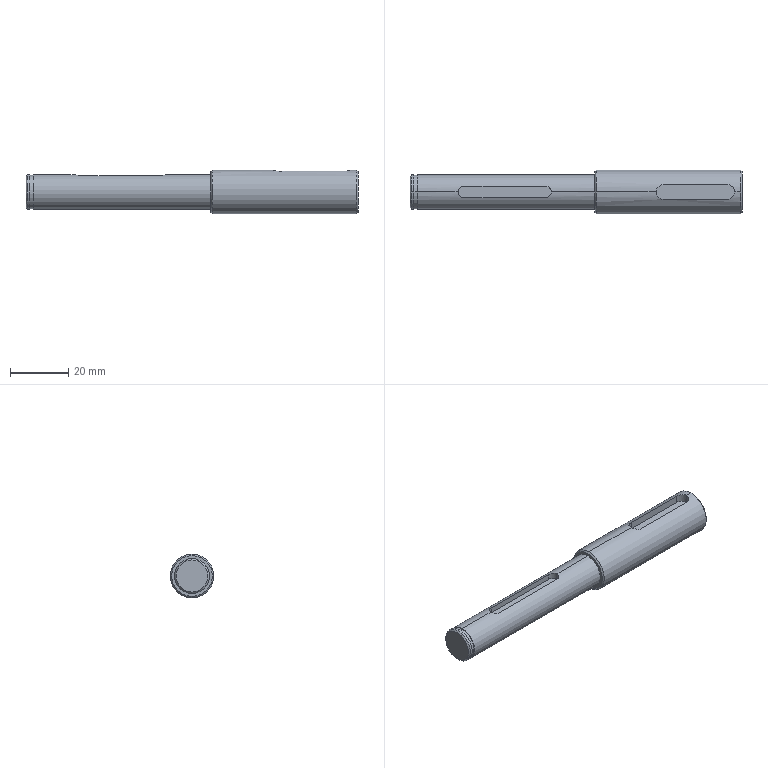Part | SolidWorks | features BaseBody 1 | 1 solid | 31 faces | box 114 x 15 x 15 mm | volume 15429 mm3 | cylinder 14 | plane 11 | cone 6 | commonest cylinder face diameters 12 x4 4 x3 5 x3 11.5 x2 15 x2
STEP:
#1=CARTESIAN_POINT('',(113.5,0.,7.5));
#2=VERTEX_POINT('',#1);
#3=CARTESIAN_POINT('',(113.5,0.,-7.5));
#4=VERTEX_POINT('',#3);
#5=CARTESIAN_POINT('',(113.5,0.,0.));
#6=DIRECTION('',(-1.,0.,0.));
#7=DIRECTION('',(0.,0.,1.));
#8=AXIS2_PLACEMENT_3D('',#5,#6,#7);
#9=CIRCLE('',#8,7.5);
#10=EDGE_CURVE('',#2,#4,#9,.T.);
#11=ORIENTED_EDGE('',*,*,#10,.T.);
#12=CARTESIAN_POINT('',(64.,0.,-7.5));
#13=VERTEX_POINT('',#12);
#14=CARTESIAN_POINT('',(0.,0.,-7.5));
#15=DIRECTION('',(-1.,0.,0.));
#16=VECTOR('',#15,1000.);
#17=LINE('',#14,#16);
#18=EDGE_CURVE('',#4,#13,#17,.T.);
#19=ORIENTED_EDGE('',*,*,#18,.T.);
#20=CARTESIAN_POINT('',(64.,0.,7.5));
#21=VERTEX_POINT('',#20);
#22=CARTESIAN_POINT('',(64.,0.,0.));
#23=DIRECTION('',(1.,0.,0.));
#24=DIRECTION('',(0.,0.,1.));
#25=AXIS2_PLACEMENT_3D('',#22,#23,#24);
#26=CIRCLE('',#25,7.5);
#27=EDGE_CURVE('',#13,#21,#26,.T.);
#28=ORIENTED_EDGE('',*,*,#27,.T.);
#29=CARTESIAN_POINT('',(84.5,0.,7.5));
#30=VERTEX_POINT('',#29);
#31=CARTESIAN_POINT('',(0.,0.,7.5));
#32=DIRECTION('',(-1.,0.,0.));
#33=VECTOR('',#32,1000.);
#34=LINE('',#31,#33);
#35=EDGE_CURVE('',#30,#21,#34,.T.);
#36=ORIENTED_EDGE('',*,*,#35,.F.);
#37=CARTESIAN_POINT('',(87.,2.5,7.071));
#38=VERTEX_POINT('',#37);
#39=CARTESIAN_POINT('',(84.5,0.,7.5));
#40=CARTESIAN_POINT('',(84.5,0.1664,7.5));
#41=CARTESIAN_POINT('',(84.516,0.3297,7.494));
#42=CARTESIAN_POINT('',(84.581,0.6507,7.473));
#43=CARTESIAN_POINT('',(84.629,0.8101,7.458));
#44=CARTESIAN_POINT('',(84.755,1.112,7.419));
#45=CARTESIAN_POINT('',(84.832,1.255,7.395));
#46=CARTESIAN_POINT('',(85.013,1.526,7.344));
#47=CARTESIAN_POINT('',(85.118,1.653,7.316));
#48=CARTESIAN_POINT('',(85.461,1.996,7.233));
#49=CARTESIAN_POINT('',(85.737,2.182,7.177));
#50=CARTESIAN_POINT('',(86.187,2.37,7.116));
#51=CARTESIAN_POINT('',(86.346,2.419,7.099));
#52=CARTESIAN_POINT('',(86.67,2.484,7.077));
#53=CARTESIAN_POINT('',(86.834,2.5,7.071));
#54=CARTESIAN_POINT('',(87.,2.5,7.071));
#55=B_SPLINE_CURVE_WITH_KNOTS('',3,(#39,#40,#41,#42,#43,#44,#45,#46,#47,#48,#49,#50,#51,#52,#53,#54),.UNSPECIFIED.,.F.,.F.,(4,2,2,2,2,2,2,4),(0.003934,0.004426,0.004917,0.005409,0.005901,0.006884,0.007376,0.007868),.UNSPECIFIED.);
#56=EDGE_CURVE('',#30,#38,#55,.T.);
#57=ORIENTED_EDGE('',*,*,#56,.T.);
#58=CARTESIAN_POINT('',(109.,2.5,7.071));
#59=VERTEX_POINT('',#58);
#60=CARTESIAN_POINT('',(0.,2.5,7.071));
#61=DIRECTION('',(1.,0.,0.));
#62=VECTOR('',#61,1000.);
#63=LINE('',#60,#62);
#64=EDGE_CURVE('',#38,#59,#63,.T.);
#65=ORIENTED_EDGE('',*,*,#64,.T.);
#66=CARTESIAN_POINT('',(111.5,0.,7.5));
#67=VERTEX_POINT('',#66);
#68=CARTESIAN_POINT('',(109.,2.5,7.071));
#69=CARTESIAN_POINT('',(109.166,2.5,7.071));
#70=CARTESIAN_POINT('',(109.33,2.484,7.077));
#71=CARTESIAN_POINT('',(109.651,2.419,7.099));
#72=CARTESIAN_POINT('',(109.81,2.371,7.116));
#73=CARTESIAN_POINT('',(110.112,2.245,7.156));
#74=CARTESIAN_POINT('',(110.255,2.168,7.18));
#75=CARTESIAN_POINT('',(110.526,1.987,7.233));
#76=CARTESIAN_POINT('',(110.653,1.883,7.261));
#77=CARTESIAN_POINT('',(110.996,1.54,7.344));
#78=CARTESIAN_POINT('',(111.182,1.263,7.399));
#79=CARTESIAN_POINT('',(111.37,0.8128,7.457));
#80=CARTESIAN_POINT('',(111.418,0.6543,7.473));
#81=CARTESIAN_POINT('',(111.484,0.3305,7.494));
#82=CARTESIAN_POINT('',(111.5,0.1664,7.5));
#83=CARTESIAN_POINT('',(111.5,0.,7.5));
#84=B_SPLINE_CURVE_WITH_KNOTS('',3,(#68,#69,#70,#71,#72,#73,#74,#75,#76,#77,#78,#79,#80,#81,#82,#83),.UNSPECIFIED.,.F.,.F.,(4,2,2,2,2,2,2,4),(-0.003934,-0.003442,-0.00295,-0.002459,-0.001967,-0.0009835,-0.0004917,0.),.UNSPECIFIED.);
#85=EDGE_CURVE('',#59,#67,#84,.T.);
#86=ORIENTED_EDGE('',*,*,#85,.T.);
#87=CARTESIAN_POINT('',(0.,0.,7.5));
#88=DIRECTION('',(-1.,0.,0.));
#89=VECTOR('',#88,1000.);
#90=LINE('',#87,#89);
#91=EDGE_CURVE('',#2,#67,#90,.T.);
#92=ORIENTED_EDGE('',*,*,#91,.F.);
#93=EDGE_LOOP('',(#11,#19,#28,#36,#57,#65,#86,#92));
#94=FACE_OUTER_BOUND('',#93,.T.);
#95=CARTESIAN_POINT('',(0.,0.,0.));
#96=DIRECTION('',(-1.,0.,0.));
#97=DIRECTION('',(0.,0.,1.));
#98=AXIS2_PLACEMENT_3D('',#95,#96,#97);
#99=CYLINDRICAL_SURFACE('',#98,7.5);
#100=ADVANCED_FACE('',(#94),#99,.T.);
#101=CARTESIAN_POINT('',(63.5,0.,-7.));
#102=VERTEX_POINT('',#101);
#103=CARTESIAN_POINT('',(63.5,0.,7.));
#104=VERTEX_POINT('',#103);
#105=CARTESIAN_POINT('',(63.5,0.,0.));
#106=DIRECTION('',(1.,0.,0.));
#107=DIRECTION('',(0.,0.,-1.));
#108=AXIS2_PLACEMENT_3D('',#105,#106,#107);
#109=CIRCLE('',#108,7.);
#110=EDGE_CURVE('',#102,#104,#109,.T.);
#111=ORIENTED_EDGE('',*,*,#110,.T.);
#112=CARTESIAN_POINT('',(64.,0.,7.5));
#113=DIRECTION('',(0.7071,0.,0.7071));
#114=VECTOR('',#113,1000.);
#115=LINE('',#112,#114);
#116=EDGE_CURVE('',#104,#21,#115,.T.);
#117=ORIENTED_EDGE('',*,*,#116,.T.);
#118=ORIENTED_EDGE('',*,*,#27,.F.);
#119=CARTESIAN_POINT('',(64.,0.,-7.5));
#120=DIRECTION('',(0.7071,0.,-0.7071));
#121=VECTOR('',#120,1000.);
#122=LINE('',#119,#121);
#123=EDGE_CURVE('',#102,#13,#122,.T.);
#124=ORIENTED_EDGE('',*,*,#123,.F.);
#125=EDGE_LOOP('',(#111,#117,#118,#124));
#126=FACE_OUTER_BOUND('',#125,.T.);
#127=CARTESIAN_POINT('',(64.,0.,0.));
#128=DIRECTION('',(1.,0.,0.));
#129=DIRECTION('',(0.,0.,-1.));
#130=AXIS2_PLACEMENT_3D('',#127,#128,#129);
#131=CONICAL_SURFACE('',#130,7.5,0.7854);
#132=ADVANCED_FACE('',(#126),#131,.T.);
#133=CARTESIAN_POINT('',(111.5,0.,4.5));
#134=VERTEX_POINT('',#133);
#135=CARTESIAN_POINT('',(109.,2.5,4.5));
#136=VERTEX_POINT('',#135);
#137=CARTESIAN_POINT('',(109.,0.,4.5));
#138=DIRECTION('',(0.,0.,1.));
#139=DIRECTION('',(1.,0.,0.));
#140=AXIS2_PLACEMENT_3D('',#137,#138,#139);
#141=CIRCLE('',#140,2.5);
#142=EDGE_CURVE('',#134,#136,#141,.T.);
#143=ORIENTED_EDGE('',*,*,#142,.F.);
#144=CARTESIAN_POINT('',(111.5,0.,4.5));
#145=DIRECTION('',(0.,0.,1.));
#146=VECTOR('',#145,1000.);
#147=LINE('',#144,#146);
#148=EDGE_CURVE('',#134,#67,#147,.T.);
#149=ORIENTED_EDGE('',*,*,#148,.T.);
#150=ORIENTED_EDGE('',*,*,#85,.F.);
#151=CARTESIAN_POINT('',(109.,2.5,4.5));
#152=DIRECTION('',(0.,0.,1.));
#153=VECTOR('',#152,1000.);
#154=LINE('',#151,#153);
#155=EDGE_CURVE('',#136,#59,#154,.T.);
#156=ORIENTED_EDGE('',*,*,#155,.F.);
#157=EDGE_LOOP('',(#143,#149,#150,#156));
#158=FACE_OUTER_BOUND('',#157,.T.);
#159=CARTESIAN_POINT('',(109.,0.,4.5));
#160=DIRECTION('',(0.,0.,1.));
#161=DIRECTION('',(1.,0.,0.));
#162=AXIS2_PLACEMENT_3D('',#159,#160,#161);
#163=CYLINDRICAL_SURFACE('',#162,2.5);
#164=ADVANCED_FACE('',(#158),#163,.F.);
#165=CARTESIAN_POINT('',(114.,0.,7.));
#166=VERTEX_POINT('',#165);
#167=CARTESIAN_POINT('',(114.,0.,-7.));
#168=VERTEX_POINT('',#167);
#169=CARTESIAN_POINT('',(114.,0.,0.));
#170=DIRECTION('',(-1.,0.,0.));
#171=DIRECTION('',(0.,0.,1.));
#172=AXIS2_PLACEMENT_3D('',#169,#170,#171);
#173=CIRCLE('',#172,7.);
#174=EDGE_CURVE('',#166,#168,#173,.T.);
#175=ORIENTED_EDGE('',*,*,#174,.T.);
#176=CARTESIAN_POINT('',(113.5,0.,-7.5));
#177=DIRECTION('',(-0.7071,0.,-0.7071));
#178=VECTOR('',#177,1000.);
#179=LINE('',#176,#178);
#180=EDGE_CURVE('',#168,#4,#179,.T.);
#181=ORIENTED_EDGE('',*,*,#180,.T.);
#182=ORIENTED_EDGE('',*,*,#10,.F.);
#183=CARTESIAN_POINT('',(113.5,0.,7.5));
#184=DIRECTION('',(-0.7071,0.,0.7071));
#185=VECTOR('',#184,1000.);
#186=LINE('',#183,#185);
#187=EDGE_CURVE('',#166,#2,#186,.T.);
#188=ORIENTED_EDGE('',*,*,#187,.F.);
#189=EDGE_LOOP('',(#175,#181,#182,#188));
#190=FACE_OUTER_BOUND('',#189,.T.);
#191=CARTESIAN_POINT('',(113.5,0.,0.));
#192=DIRECTION('',(-1.,0.,0.));
#193=DIRECTION('',(0.,0.,1.));
#194=AXIS2_PLACEMENT_3D('',#191,#192,#193);
#195=CONICAL_SURFACE('',#194,7.5,0.7854);
#196=ADVANCED_FACE('',(#190),#195,.T.);
#197=CARTESIAN_POINT('',(63.5,0.,6.));
#198=VERTEX_POINT('',#197);
#199=CARTESIAN_POINT('',(63.5,0.,-6.));
#200=VERTEX_POINT('',#199);
#201=CARTESIAN_POINT('',(63.5,0.,0.));
#202=DIRECTION('',(-1.,0.,0.));
#203=DIRECTION('',(0.,0.,1.));
#204=AXIS2_PLACEMENT_3D('',#201,#202,#203);
#205=CIRCLE('',#204,6.);
#206=EDGE_CURVE('',#198,#200,#205,.T.);
#207=ORIENTED_EDGE('',*,*,#206,.T.);
#208=CARTESIAN_POINT('',(2.5,0.,-6.));
#209=VERTEX_POINT('',#208);
#210=CARTESIAN_POINT('',(0.,0.,-6.));
#211=DIRECTION('',(-1.,0.,0.));
#212=VECTOR('',#211,1000.);
#213=LINE('',#210,#212);
#214=EDGE_CURVE('',#200,#209,#213,.T.);
#215=ORIENTED_EDGE('',*,*,#214,.T.);
#216=CARTESIAN_POINT('',(2.5,0.,6.));
#217=VERTEX_POINT('',#216);
#218=CARTESIAN_POINT('',(2.5,0.,0.));
#219=DIRECTION('',(1.,0.,0.));
#220=DIRECTION('',(0.,0.,1.));
#221=AXIS2_PLACEMENT_3D('',#218,#219,#220);
#222=CIRCLE('',#221,6.);
#223=EDGE_CURVE('',#209,#217,#222,.T.);
#224=ORIENTED_EDGE('',*,*,#223,.T.);
#225=CARTESIAN_POINT('',(16.5,0.,6.));
#226=VERTEX_POINT('',#225);
#227=CARTESIAN_POINT('',(0.,0.,6.));
#228=DIRECTION('',(-1.,0.,0.));
#229=VECTOR('',#228,1000.);
#230=LINE('',#227,#229);
#231=EDGE_CURVE('',#226,#217,#230,.T.);
#232=ORIENTED_EDGE('',*,*,#231,.F.);
#233=CARTESIAN_POINT('',(18.5,2.,5.657));
#234=VERTEX_POINT('',#233);
#235=CARTESIAN_POINT('',(16.5,0.,6.));
#236=CARTESIAN_POINT('',(16.5,0.1331,6.));
#237=CARTESIAN_POINT('',(16.513,0.2638,5.996));
#238=CARTESIAN_POINT('',(16.565,0.5206,5.979));
#239=CARTESIAN_POINT('',(16.603,0.6481,5.966));
#240=CARTESIAN_POINT('',(16.704,0.8898,5.935));
#241=CARTESIAN_POINT('',(16.766,1.004,5.916));
#242=CARTESIAN_POINT('',(16.911,1.221,5.876));
#243=CARTESIAN_POINT('',(16.994,1.323,5.853));
#244=CARTESIAN_POINT('',(17.269,1.597,5.787));
#245=CARTESIAN_POINT('',(17.49,1.746,5.741));
#246=CARTESIAN_POINT('',(17.85,1.896,5.693));
#247=CARTESIAN_POINT('',(17.977,1.935,5.68));
#248=CARTESIAN_POINT('',(18.236,1.987,5.662));
#249=CARTESIAN_POINT('',(18.367,2.,5.657));
#250=CARTESIAN_POINT('',(18.5,2.,5.657));
#251=B_SPLINE_CURVE_WITH_KNOTS('',3,(#235,#236,#237,#238,#239,#240,#241,#242,#243,#244,#245,#246,#247,#248,#249,#250),.UNSPECIFIED.,.F.,.F.,(4,2,2,2,2,2,2,4),(0.,0.0003934,0.0007868,0.00118,0.001574,0.00236,0.002754,0.003147),.UNSPECIFIED.);
#252=EDGE_CURVE('',#226,#234,#251,.T.);
#253=ORIENTED_EDGE('',*,*,#252,.T.);
#254=CARTESIAN_POINT('',(46.5,2.,5.657));
#255=VERTEX_POINT('',#254);
#256=CARTESIAN_POINT('',(0.,2.,5.657));
#257=DIRECTION('',(1.,0.,0.));
#258=VECTOR('',#257,1000.);
#259=LINE('',#256,#258);
#260=EDGE_CURVE('',#234,#255,#259,.T.);
#261=ORIENTED_EDGE('',*,*,#260,.T.);
#262=CARTESIAN_POINT('',(48.5,0.,6.));
#263=VERTEX_POINT('',#262);
#264=CARTESIAN_POINT('',(46.5,2.,5.657));
#265=CARTESIAN_POINT('',(46.633,2.,5.657));
#266=CARTESIAN_POINT('',(46.764,1.987,5.662));
#267=CARTESIAN_POINT('',(47.021,1.936,5.679));
#268=CARTESIAN_POINT('',(47.148,1.897,5.693));
#269=CARTESIAN_POINT('',(47.39,1.796,5.725));
#270=CARTESIAN_POINT('',(47.504,1.735,5.744));
#271=CARTESIAN_POINT('',(47.721,1.59,5.786));
#272=CARTESIAN_POINT('',(47.822,1.506,5.809));
#273=CARTESIAN_POINT('',(48.097,1.232,5.875));
#274=CARTESIAN_POINT('',(48.245,1.01,5.919));
#275=CARTESIAN_POINT('',(48.396,0.6502,5.966));
#276=CARTESIAN_POINT('',(48.435,0.5235,5.979));
#277=CARTESIAN_POINT('',(48.487,0.2644,5.996));
#278=CARTESIAN_POINT('',(48.5,0.1331,6.));
#279=CARTESIAN_POINT('',(48.5,0.,6.));
#280=B_SPLINE_CURVE_WITH_KNOTS('',3,(#264,#265,#266,#267,#268,#269,#270,#271,#272,#273,#274,#275,#276,#277,#278,#279),.UNSPECIFIED.,.F.,.F.,(4,2,2,2,2,2,2,4),(0.,0.0003934,0.0007868,0.00118,0.001574,0.00236,0.002754,0.003147),.UNSPECIFIED.);
#281=EDGE_CURVE('',#255,#263,#280,.T.);
#282=ORIENTED_EDGE('',*,*,#281,.T.);
#283=CARTESIAN_POINT('',(0.,0.,6.));
#284=DIRECTION('',(-1.,0.,0.));
#285=VECTOR('',#284,1000.);
#286=LINE('',#283,#285);
#287=EDGE_CURVE('',#198,#263,#286,.T.);
#288=ORIENTED_EDGE('',*,*,#287,.F.);
#289=EDGE_LOOP('',(#207,#215,#224,#232,#253,#261,#282,#288));
#290=FACE_OUTER_BOUND('',#289,.T.);
#291=CARTESIAN_POINT('',(0.,0.,0.));
#292=DIRECTION('',(-1.,0.,0.));
#293=DIRECTION('',(0.,0.,1.));
#294=AXIS2_PLACEMENT_3D('',#291,#292,#293);
#295=CYLINDRICAL_SURFACE('',#294,6.);
#296=ADVANCED_FACE('',(#290),#295,.T.);
#297=CARTESIAN_POINT('',(48.5,0.,3.65));
#298=VERTEX_POINT('',#297);
#299=CARTESIAN_POINT('',(46.5,2.,3.65));
#300=VERTEX_POINT('',#299);
#301=CARTESIAN_POINT('',(46.5,0.,3.65));
#302=DIRECTION('',(0.,0.,1.));
#303=DIRECTION('',(1.,0.,0.));
#304=AXIS2_PLACEMENT_3D('',#301,#302,#303);
#305=CIRCLE('',#304,2.);
#306=EDGE_CURVE('',#298,#300,#305,.T.);
#307=ORIENTED_EDGE('',*,*,#306,.F.);
#308=CARTESIAN_POINT('',(48.5,0.,3.65));
#309=DIRECTION('',(0.,0.,1.));
#310=VECTOR('',#309,1000.);
#311=LINE('',#308,#310);
#312=EDGE_CURVE('',#298,#263,#311,.T.);
#313=ORIENTED_EDGE('',*,*,#312,.T.);
#314=ORIENTED_EDGE('',*,*,#281,.F.);
#315=CARTESIAN_POINT('',(46.5,2.,3.65));
#316=DIRECTION('',(0.,0.,1.));
#317=VECTOR('',#316,1000.);
#318=LINE('',#315,#317);
#319=EDGE_CURVE('',#300,#255,#318,.T.);
#320=ORIENTED_EDGE('',*,*,#319,.F.);
#321=EDGE_LOOP('',(#307,#313,#314,#320));
#322=FACE_OUTER_BOUND('',#321,.T.);
#323=CARTESIAN_POINT('',(46.5,0.,3.65));
#324=DIRECTION('',(0.,0.,1.));
#325=DIRECTION('',(1.,0.,0.));
#326=AXIS2_PLACEMENT_3D('',#323,#324,#325);
#327=CYLINDRICAL_SURFACE('',#326,2.);
#328=ADVANCED_FACE('',(#322),#327,.F.);
#329=CARTESIAN_POINT('',(2.5,0.,5.75));
#330=VERTEX_POINT('',#329);
#331=CARTESIAN_POINT('',(2.5,0.,-5.75));
#332=VERTEX_POINT('',#331);
#333=CARTESIAN_POINT('',(2.5,0.,0.));
#334=DIRECTION('',(-1.,0.,0.));
#335=DIRECTION('',(0.,0.,1.));
#336=AXIS2_PLACEMENT_3D('',#333,#334,#335);
#337=CIRCLE('',#336,5.75);
#338=EDGE_CURVE('',#330,#332,#337,.T.);
#339=ORIENTED_EDGE('',*,*,#338,.T.);
#340=CARTESIAN_POINT('',(1.35,0.,-5.75));
#341=VERTEX_POINT('',#340);
#342=CARTESIAN_POINT('',(0.,0.,-5.75));
#343=DIRECTION('',(-1.,0.,0.));
#344=VECTOR('',#343,1000.);
#345=LINE('',#342,#344);
#346=EDGE_CURVE('',#332,#341,#345,.T.);
#347=ORIENTED_EDGE('',*,*,#346,.T.);
#348=CARTESIAN_POINT('',(1.35,0.,5.75));
#349=VERTEX_POINT('',#348);
#350=CARTESIAN_POINT('',(1.35,0.,0.));
#351=DIRECTION('',(1.,0.,0.));
#352=DIRECTION('',(0.,0.,1.));
#353=AXIS2_PLACEMENT_3D('',#350,#351,#352);
#354=CIRCLE('',#353,5.75);
#355=EDGE_CURVE('',#341,#349,#354,.T.);
#356=ORIENTED_EDGE('',*,*,#355,.T.);
#357=CARTESIAN_POINT('',(0.,0.,5.75));
#358=DIRECTION('',(-1.,0.,0.));
#359=VECTOR('',#358,1000.);
#360=LINE('',#357,#359);
#361=EDGE_CURVE('',#330,#349,#360,.T.);
#362=ORIENTED_EDGE('',*,*,#361,.F.);
#363=EDGE_LOOP('',(#339,#347,#356,#362));
#364=FACE_OUTER_BOUND('',#363,.T.);
#365=CARTESIAN_POINT('',(0.,0.,0.));
#366=DIRECTION('',(-1.,0.,0.));
#367=DIRECTION('',(0.,0.,1.));
#368=AXIS2_PLACEMENT_3D('',#365,#366,#367);
#369=CYLINDRICAL_SURFACE('',#368,5.75);
#370=ADVANCED_FACE('',(#364),#369,.T.);
#371=CARTESIAN_POINT('',(1.35,0.,6.));
#372=VERTEX_POINT('',#371);
#373=CARTESIAN_POINT('',(1.35,0.,-6.));
#374=VERTEX_POINT('',#373);
#375=CARTESIAN_POINT('',(1.35,0.,0.));
#376=DIRECTION('',(-1.,0.,0.));
#377=DIRECTION('',(0.,0.,1.));
#378=AXIS2_PLACEMENT_3D('',#375,#376,#377);
#379=CIRCLE('',#378,6.);
#380=EDGE_CURVE('',#372,#374,#379,.T.);
#381=ORIENTED_EDGE('',*,*,#380,.T.);
#382=CARTESIAN_POINT('',(0.5,0.,-6.));
#383=VERTEX_POINT('',#382);
#384=CARTESIAN_POINT('',(0.,0.,-6.));
#385=DIRECTION('',(-1.,0.,0.));
#386=VECTOR('',#385,1000.);
#387=LINE('',#384,#386);
#388=EDGE_CURVE('',#374,#383,#387,.T.);
#389=ORIENTED_EDGE('',*,*,#388,.T.);
#390=CARTESIAN_POINT('',(0.5,0.,6.));
#391=VERTEX_POINT('',#390);
#392=CARTESIAN_POINT('',(0.5,0.,0.));
#393=DIRECTION('',(1.,0.,0.));
#394=DIRECTION('',(0.,0.,1.));
#395=AXIS2_PLACEMENT_3D('',#392,#393,#394);
#396=CIRCLE('',#395,6.);
#397=EDGE_CURVE('',#383,#391,#396,.T.);
#398=ORIENTED_EDGE('',*,*,#397,.T.);
#399=CARTESIAN_POINT('',(0.,0.,6.));
#400=DIRECTION('',(-1.,0.,0.));
#401=VECTOR('',#400,1000.);
#402=LINE('',#399,#401);
#403=EDGE_CURVE('',#372,#391,#402,.T.);
#404=ORIENTED_EDGE('',*,*,#403,.F.);
#405=EDGE_LOOP('',(#381,#389,#398,#404));
#406=FACE_OUTER_BOUND('',#405,.T.);
#407=CARTESIAN_POINT('',(0.,0.,0.));
#408=DIRECTION('',(-1.,0.,0.));
#409=DIRECTION('',(0.,0.,1.));
#410=AXIS2_PLACEMENT_3D('',#407,#408,#409);
#411=CYLINDRICAL_SURFACE('',#410,6.);
#412=ADVANCED_FACE('',(#406),#411,.T.);
#413=CARTESIAN_POINT('',(0.,0.,-5.5));
#414=VERTEX_POINT('',#413);
#415=CARTESIAN_POINT('',(0.,0.,5.5));
#416=VERTEX_POINT('',#415);
#417=CARTESIAN_POINT('',(0.,0.,0.));
#418=DIRECTION('',(1.,0.,0.));
#419=DIRECTION('',(0.,0.,-1.));
#420=AXIS2_PLACEMENT_3D('',#417,#418,#419);
#421=CIRCLE('',#420,5.5);
#422=EDGE_CURVE('',#414,#416,#421,.T.);
#423=ORIENTED_EDGE('',*,*,#422,.T.);
#424=CARTESIAN_POINT('',(0.5,0.,6.));
#425=DIRECTION('',(0.7071,0.,0.7071));
#426=VECTOR('',#425,1000.);
#427=LINE('',#424,#426);
#428=EDGE_CURVE('',#416,#391,#427,.T.);
#429=ORIENTED_EDGE('',*,*,#428,.T.);
#430=ORIENTED_EDGE('',*,*,#397,.F.);
#431=CARTESIAN_POINT('',(0.5,0.,-6.));
#432=DIRECTION('',(0.7071,0.,-0.7071));
#433=VECTOR('',#432,1000.);
#434=LINE('',#431,#433);
#435=EDGE_CURVE('',#414,#383,#434,.T.);
#436=ORIENTED_EDGE('',*,*,#435,.F.);
#437=EDGE_LOOP('',(#423,#429,#430,#436));
#438=FACE_OUTER_BOUND('',#437,.T.);
#439=CARTESIAN_POINT('',(0.5,0.,0.));
#440=DIRECTION('',(1.,0.,0.));
#441=DIRECTION('',(0.,0.,-1.));
#442=AXIS2_PLACEMENT_3D('',#439,#440,#441);
#443=CONICAL_SURFACE('',#442,6.,0.7854);
#444=ADVANCED_FACE('',(#438),#443,.T.);
#445=ORIENTED_EDGE('',*,*,#18,.F.);
#446=CARTESIAN_POINT('',(113.5,0.,0.));
#447=DIRECTION('',(-1.,0.,0.));
#448=DIRECTION('',(0.,0.,1.));
#449=AXIS2_PLACEMENT_3D('',#446,#447,#448);
#450=CIRCLE('',#449,7.5);
#451=EDGE_CURVE('',#4,#2,#450,.T.);
#452=ORIENTED_EDGE('',*,*,#451,.T.);
#453=ORIENTED_EDGE('',*,*,#91,.T.);
#454=CARTESIAN_POINT('',(109.,-2.5,7.071));
#455=VERTEX_POINT('',#454);
#456=CARTESIAN_POINT('',(111.5,0.,7.5));
#457=CARTESIAN_POINT('',(111.5,-0.1664,7.5));
#458=CARTESIAN_POINT('',(111.484,-0.3297,7.494));
#459=CARTESIAN_POINT('',(111.419,-0.6507,7.473));
#460=CARTESIAN_POINT('',(111.371,-0.8101,7.458));
#461=CARTESIAN_POINT('',(111.245,-1.112,7.419));
#462=CARTESIAN_POINT('',(111.168,-1.255,7.395));
#463=CARTESIAN_POINT('',(110.987,-1.526,7.344));
#464=CARTESIAN_POINT('',(110.882,-1.653,7.316));
#465=CARTESIAN_POINT('',(110.539,-1.996,7.233));
#466=CARTESIAN_POINT('',(110.263,-2.182,7.177));
#467=CARTESIAN_POINT('',(109.813,-2.37,7.116));
#468=CARTESIAN_POINT('',(109.654,-2.419,7.099));
#469=CARTESIAN_POINT('',(109.33,-2.484,7.077));
#470=CARTESIAN_POINT('',(109.166,-2.5,7.071));
#471=CARTESIAN_POINT('',(109.,-2.5,7.071));
#472=B_SPLINE_CURVE_WITH_KNOTS('',3,(#456,#457,#458,#459,#460,#461,#462,#463,#464,#465,#466,#467,#468,#469,#470,#471),.UNSPECIFIED.,.F.,.F.,(4,2,2,2,2,2,2,4),(0.,0.0004917,0.0009835,0.001475,0.001967,0.00295,0.003442,0.003934),.UNSPECIFIED.);
#473=EDGE_CURVE('',#67,#455,#472,.T.);
#474=ORIENTED_EDGE('',*,*,#473,.T.);
#475=CARTESIAN_POINT('',(87.,-2.5,7.071));
#476=VERTEX_POINT('',#475);
#477=CARTESIAN_POINT('',(0.,-2.5,7.071));
#478=DIRECTION('',(-1.,0.,0.));
#479=VECTOR('',#478,1000.);
#480=LINE('',#477,#479);
#481=EDGE_CURVE('',#455,#476,#480,.T.);
#482=ORIENTED_EDGE('',*,*,#481,.T.);
#483=CARTESIAN_POINT('',(87.,-2.5,7.071));
#484=CARTESIAN_POINT('',(86.834,-2.5,7.071));
#485=CARTESIAN_POINT('',(86.67,-2.484,7.077));
#486=CARTESIAN_POINT('',(86.349,-2.419,7.099));
#487=CARTESIAN_POINT('',(86.19,-2.371,7.116));
#488=CARTESIAN_POINT('',(85.888,-2.245,7.156));
#489=CARTESIAN_POINT('',(85.745,-2.168,7.18));
#490=CARTESIAN_POINT('',(85.474,-1.987,7.233));
#491=CARTESIAN_POINT('',(85.347,-1.883,7.261));
#492=CARTESIAN_POINT('',(85.004,-1.54,7.344));
#493=CARTESIAN_POINT('',(84.818,-1.263,7.399));
#494=CARTESIAN_POINT('',(84.63,-0.8128,7.457));
#495=CARTESIAN_POINT('',(84.582,-0.6543,7.473));
#496=CARTESIAN_POINT('',(84.516,-0.3305,7.494));
#497=CARTESIAN_POINT('',(84.5,-0.1664,7.5));
#498=CARTESIAN_POINT('',(84.5,0.,7.5));
#499=B_SPLINE_CURVE_WITH_KNOTS('',3,(#483,#484,#485,#486,#487,#488,#489,#490,#491,#492,#493,#494,#495,#496,#497,#498),.UNSPECIFIED.,.F.,.F.,(4,2,2,2,2,2,2,4),(0.,0.0004917,0.0009834,0.001475,0.001967,0.00295,0.003442,0.003934),.UNSPECIFIED.);
#500=EDGE_CURVE('',#476,#30,#499,.T.);
#501=ORIENTED_EDGE('',*,*,#500,.T.);
#502=ORIENTED_EDGE('',*,*,#35,.T.);
#503=CARTESIAN_POINT('',(64.,0.,0.));
#504=DIRECTION('',(1.,0.,0.));
#505=DIRECTION('',(0.,0.,1.));
#506=AXIS2_PLACEMENT_3D('',#503,#504,#505);
#507=CIRCLE('',#506,7.5);
#508=EDGE_CURVE('',#21,#13,#507,.T.);
#509=ORIENTED_EDGE('',*,*,#508,.T.);
#510=EDGE_LOOP('',(#445,#452,#453,#474,#482,#501,#502,#509));
#511=FACE_OUTER_BOUND('',#510,.T.);
#512=CARTESIAN_POINT('',(0.,0.,0.));
#513=DIRECTION('',(-1.,0.,0.));
#514=DIRECTION('',(0.,0.,1.));
#515=AXIS2_PLACEMENT_3D('',#512,#513,#514);
#516=CYLINDRICAL_SURFACE('',#515,7.5);
#517=ADVANCED_FACE('',(#511),#516,.T.);
#518=ORIENTED_EDGE('',*,*,#116,.F.);
#519=CARTESIAN_POINT('',(63.5,0.,0.));
#520=DIRECTION('',(1.,0.,0.));
#521=DIRECTION('',(0.,0.,-1.));
#522=AXIS2_PLACEMENT_3D('',#519,#520,#521);
#523=CIRCLE('',#522,7.);
#524=EDGE_CURVE('',#104,#102,#523,.T.);
#525=ORIENTED_EDGE('',*,*,#524,.T.);
#526=ORIENTED_EDGE('',*,*,#123,.T.);
#527=ORIENTED_EDGE('',*,*,#508,.F.);
#528=EDGE_LOOP('',(#518,#525,#526,#527));
#529=FACE_OUTER_BOUND('',#528,.T.);
#530=CARTESIAN_POINT('',(64.,0.,0.));
#531=DIRECTION('',(1.,0.,0.));
#532=DIRECTION('',(0.,0.,-1.));
#533=AXIS2_PLACEMENT_3D('',#530,#531,#532);
#534=CONICAL_SURFACE('',#533,7.5,0.7854);
#535=ADVANCED_FACE('',(#529),#534,.T.);
#536=CARTESIAN_POINT('',(87.,2.5,4.5));
#537=VERTEX_POINT('',#536);
#538=CARTESIAN_POINT('',(87.,-2.5,4.5));
#539=VERTEX_POINT('',#538);
#540=CARTESIAN_POINT('',(87.,0.,4.5));
#541=DIRECTION('',(0.,0.,1.));
#542=DIRECTION('',(1.,0.,0.));
#543=AXIS2_PLACEMENT_3D('',#540,#541,#542);
#544=CIRCLE('',#543,2.5);
#545=EDGE_CURVE('',#537,#539,#544,.T.);
#546=ORIENTED_EDGE('',*,*,#545,.F.);
#547=CARTESIAN_POINT('',(87.,2.5,4.5));
#548=DIRECTION('',(0.,0.,-1.));
#549=VECTOR('',#548,1000.);
#550=LINE('',#547,#549);
#551=EDGE_CURVE('',#38,#537,#550,.T.);
#552=ORIENTED_EDGE('',*,*,#551,.F.);
#553=ORIENTED_EDGE('',*,*,#56,.F.);
#554=ORIENTED_EDGE('',*,*,#500,.F.);
#555=CARTESIAN_POINT('',(87.,-2.5,4.5));
#556=DIRECTION('',(0.,0.,1.));
#557=VECTOR('',#556,1000.);
#558=LINE('',#555,#557);
#559=EDGE_CURVE('',#539,#476,#558,.T.);
#560=ORIENTED_EDGE('',*,*,#559,.F.);
#561=EDGE_LOOP('',(#546,#552,#553,#554,#560));
#562=FACE_OUTER_BOUND('',#561,.T.);
#563=CARTESIAN_POINT('',(87.,0.,4.5));
#564=DIRECTION('',(0.,0.,1.));
#565=DIRECTION('',(1.,0.,0.));
#566=AXIS2_PLACEMENT_3D('',#563,#564,#565);
#567=CYLINDRICAL_SURFACE('',#566,2.5);
#568=ADVANCED_FACE('',(#562),#567,.F.);
#569=CARTESIAN_POINT('',(109.,-2.5,4.5));
#570=VERTEX_POINT('',#569);
#571=CARTESIAN_POINT('',(87.,-2.5,4.5));
#572=DIRECTION('',(1.,0.,0.));
#573=VECTOR('',#572,1000.);
#574=LINE('',#571,#573);
#575=EDGE_CURVE('',#539,#570,#574,.T.);
#576=ORIENTED_EDGE('',*,*,#575,.F.);
#577=ORIENTED_EDGE('',*,*,#559,.T.);
#578=ORIENTED_EDGE('',*,*,#481,.F.);
#579=CARTESIAN_POINT('',(109.,-2.5,4.5));
#580=DIRECTION('',(0.,0.,1.));
#581=VECTOR('',#580,1000.);
#582=LINE('',#579,#581);
#583=EDGE_CURVE('',#570,#455,#582,.T.);
#584=ORIENTED_EDGE('',*,*,#583,.F.);
#585=EDGE_LOOP('',(#576,#577,#578,#584));
#586=FACE_OUTER_BOUND('',#585,.T.);
#587=CARTESIAN_POINT('',(87.,-2.5,4.5));
#588=DIRECTION('',(0.,-1.,0.));
#589=DIRECTION('',(1.,0.,0.));
#590=AXIS2_PLACEMENT_3D('',#587,#588,#589);
#591=PLANE('',#590);
#592=ADVANCED_FACE('',(#586),#591,.F.);
#593=ORIENTED_EDGE('',*,*,#148,.F.);
#594=CARTESIAN_POINT('',(109.,0.,4.5));
#595=DIRECTION('',(0.,0.,1.));
#596=DIRECTION('',(1.,0.,0.));
#597=AXIS2_PLACEMENT_3D('',#594,#595,#596);
#598=CIRCLE('',#597,2.5);
#599=EDGE_CURVE('',#570,#134,#598,.T.);
#600=ORIENTED_EDGE('',*,*,#599,.F.);
#601=ORIENTED_EDGE('',*,*,#583,.T.);
#602=ORIENTED_EDGE('',*,*,#473,.F.);
#603=EDGE_LOOP('',(#593,#600,#601,#602));
#604=FACE_OUTER_BOUND('',#603,.T.);
#605=CARTESIAN_POINT('',(109.,0.,4.5));
#606=DIRECTION('',(0.,0.,1.));
#607=DIRECTION('',(1.,0.,0.));
#608=AXIS2_PLACEMENT_3D('',#605,#606,#607);
#609=CYLINDRICAL_SURFACE('',#608,2.5);
#610=ADVANCED_FACE('',(#604),#609,.F.);
#611=ORIENTED_EDGE('',*,*,#180,.F.);
#612=CARTESIAN_POINT('',(114.,0.,0.));
#613=DIRECTION('',(-1.,0.,0.));
#614=DIRECTION('',(0.,0.,1.));
#615=AXIS2_PLACEMENT_3D('',#612,#613,#614);
#616=CIRCLE('',#615,7.);
#617=EDGE_CURVE('',#168,#166,#616,.T.);
#618=ORIENTED_EDGE('',*,*,#617,.T.);
#619=ORIENTED_EDGE('',*,*,#187,.T.);
#620=ORIENTED_EDGE('',*,*,#451,.F.);
#621=EDGE_LOOP('',(#611,#618,#619,#620));
#622=FACE_OUTER_BOUND('',#621,.T.);
#623=CARTESIAN_POINT('',(113.5,0.,0.));
#624=DIRECTION('',(-1.,0.,0.));
#625=DIRECTION('',(0.,0.,1.));
#626=AXIS2_PLACEMENT_3D('',#623,#624,#625);
#627=CONICAL_SURFACE('',#626,7.5,0.7854);
#628=ADVANCED_FACE('',(#622),#627,.T.);
#629=ORIENTED_EDGE('',*,*,#206,.F.);
#630=CARTESIAN_POINT('',(63.5,0.,0.));
#631=DIRECTION('',(-1.,0.,0.));
#632=DIRECTION('',(0.,0.,1.));
#633=AXIS2_PLACEMENT_3D('',#630,#631,#632);
#634=CIRCLE('',#633,6.);
#635=EDGE_CURVE('',#200,#198,#634,.T.);
#636=ORIENTED_EDGE('',*,*,#635,.F.);
#637=EDGE_LOOP('',(#629,#636));
#638=FACE_BOUND('',#637,.T.);
#639=ORIENTED_EDGE('',*,*,#110,.F.);
#640=ORIENTED_EDGE('',*,*,#524,.F.);
#641=EDGE_LOOP('',(#639,#640));
#642=FACE_OUTER_BOUND('',#641,.T.);
#643=CARTESIAN_POINT('',(63.5,6.,0.));
#644=DIRECTION('',(1.,0.,0.));
#645=DIRECTION('',(0.,0.,-1.));
#646=AXIS2_PLACEMENT_3D('',#643,#644,#645);
#647=PLANE('',#646);
#648=ADVANCED_FACE('',(#638,#642),#647,.F.);
#649=CARTESIAN_POINT('',(87.,2.5,4.5));
#650=DIRECTION('',(-1.,0.,0.));
#651=VECTOR('',#650,1000.);
#652=LINE('',#649,#651);
#653=EDGE_CURVE('',#136,#537,#652,.T.);
#654=ORIENTED_EDGE('',*,*,#653,.F.);
#655=ORIENTED_EDGE('',*,*,#155,.T.);
#656=ORIENTED_EDGE('',*,*,#64,.F.);
#657=ORIENTED_EDGE('',*,*,#551,.T.);
#658=EDGE_LOOP('',(#654,#655,#656,#657));
#659=FACE_OUTER_BOUND('',#658,.T.);
#660=CARTESIAN_POINT('',(87.,2.5,4.5));
#661=DIRECTION('',(0.,1.,0.));
#662=DIRECTION('',(-1.,0.,0.));
#663=AXIS2_PLACEMENT_3D('',#660,#661,#662);
#664=PLANE('',#663);
#665=ADVANCED_FACE('',(#659),#664,.F.);
#666=ORIENTED_EDGE('',*,*,#599,.T.);
#667=ORIENTED_EDGE('',*,*,#142,.T.);
#668=ORIENTED_EDGE('',*,*,#653,.T.);
#669=ORIENTED_EDGE('',*,*,#545,.T.);
#670=ORIENTED_EDGE('',*,*,#575,.T.);
#671=EDGE_LOOP('',(#666,#667,#668,#669,#670));
#672=FACE_OUTER_BOUND('',#671,.T.);
#673=CARTESIAN_POINT('',(87.,0.,4.5));
#674=DIRECTION('',(0.,0.,1.));
#675=DIRECTION('',(1.,0.,0.));
#676=AXIS2_PLACEMENT_3D('',#673,#674,#675);
#677=PLANE('',#676);
#678=ADVANCED_FACE('',(#672),#677,.T.);
#679=ORIENTED_EDGE('',*,*,#174,.F.);
#680=ORIENTED_EDGE('',*,*,#617,.F.);
#681=EDGE_LOOP('',(#679,#680));
#682=FACE_OUTER_BOUND('',#681,.T.);
#683=CARTESIAN_POINT('',(114.,7.5,0.));
#684=DIRECTION('',(-1.,0.,0.));
#685=DIRECTION('',(0.,0.,1.));
#686=AXIS2_PLACEMENT_3D('',#683,#684,#685);
#687=PLANE('',#686);
#688=ADVANCED_FACE('',(#682),#687,.F.);
#689=ORIENTED_EDGE('',*,*,#214,.F.);
#690=ORIENTED_EDGE('',*,*,#635,.T.);
#691=ORIENTED_EDGE('',*,*,#287,.T.);
#692=CARTESIAN_POINT('',(46.5,-2.,5.657));
#693=VERTEX_POINT('',#692);
#694=CARTESIAN_POINT('',(48.5,0.,6.));
#695=CARTESIAN_POINT('',(48.5,-0.1331,6.));
#696=CARTESIAN_POINT('',(48.487,-0.2638,5.996));
#697=CARTESIAN_POINT('',(48.435,-0.5206,5.979));
#698=CARTESIAN_POINT('',(48.397,-0.6481,5.966));
#699=CARTESIAN_POINT('',(48.296,-0.8898,5.935));
#700=CARTESIAN_POINT('',(48.234,-1.004,5.916));
#701=CARTESIAN_POINT('',(48.089,-1.221,5.876));
#702=CARTESIAN_POINT('',(48.006,-1.323,5.853));
#703=CARTESIAN_POINT('',(47.731,-1.597,5.787));
#704=CARTESIAN_POINT('',(47.51,-1.746,5.741));
#705=CARTESIAN_POINT('',(47.15,-1.896,5.693));
#706=CARTESIAN_POINT('',(47.023,-1.935,5.68));
#707=CARTESIAN_POINT('',(46.764,-1.987,5.662));
#708=CARTESIAN_POINT('',(46.633,-2.,5.657));
#709=CARTESIAN_POINT('',(46.5,-2.,5.657));
#710=B_SPLINE_CURVE_WITH_KNOTS('',3,(#694,#695,#696,#697,#698,#699,#700,#701,#702,#703,#704,#705,#706,#707,#708,#709),.UNSPECIFIED.,.F.,.F.,(4,2,2,2,2,2,2,4),(0.003147,0.00354,0.003934,0.004327,0.004721,0.005507,0.005901,0.006294),.UNSPECIFIED.);
#711=EDGE_CURVE('',#263,#693,#710,.T.);
#712=ORIENTED_EDGE('',*,*,#711,.T.);
#713=CARTESIAN_POINT('',(18.5,-2.,5.657));
#714=VERTEX_POINT('',#713);
#715=CARTESIAN_POINT('',(0.,-2.,5.657));
#716=DIRECTION('',(-1.,0.,0.));
#717=VECTOR('',#716,1000.);
#718=LINE('',#715,#717);
#719=EDGE_CURVE('',#693,#714,#718,.T.);
#720=ORIENTED_EDGE('',*,*,#719,.T.);
#721=CARTESIAN_POINT('',(18.5,-2.,5.657));
#722=CARTESIAN_POINT('',(18.367,-2.,5.657));
#723=CARTESIAN_POINT('',(18.236,-1.987,5.662));
#724=CARTESIAN_POINT('',(17.979,-1.936,5.679));
#725=CARTESIAN_POINT('',(17.852,-1.897,5.693));
#726=CARTESIAN_POINT('',(17.61,-1.796,5.725));
#727=CARTESIAN_POINT('',(17.496,-1.735,5.744));
#728=CARTESIAN_POINT('',(17.279,-1.59,5.786));
#729=CARTESIAN_POINT('',(17.178,-1.506,5.809));
#730=CARTESIAN_POINT('',(16.903,-1.232,5.875));
#731=CARTESIAN_POINT('',(16.755,-1.01,5.919));
#732=CARTESIAN_POINT('',(16.604,-0.6502,5.966));
#733=CARTESIAN_POINT('',(16.565,-0.5235,5.979));
#734=CARTESIAN_POINT('',(16.513,-0.2644,5.996));
#735=CARTESIAN_POINT('',(16.5,-0.1331,6.));
#736=CARTESIAN_POINT('',(16.5,0.,6.));
#737=B_SPLINE_CURVE_WITH_KNOTS('',3,(#721,#722,#723,#724,#725,#726,#727,#728,#729,#730,#731,#732,#733,#734,#735,#736),.UNSPECIFIED.,.F.,.F.,(4,2,2,2,2,2,2,4),(-0.003147,-0.002754,-0.00236,-0.001967,-0.001574,-0.0007868,-0.0003934,0.),.UNSPECIFIED.);
#738=EDGE_CURVE('',#714,#226,#737,.T.);
#739=ORIENTED_EDGE('',*,*,#738,.T.);
#740=ORIENTED_EDGE('',*,*,#231,.T.);
#741=CARTESIAN_POINT('',(2.5,0.,0.));
#742=DIRECTION('',(1.,0.,0.));
#743=DIRECTION('',(0.,0.,1.));
#744=AXIS2_PLACEMENT_3D('',#741,#742,#743);
#745=CIRCLE('',#744,6.);
#746=EDGE_CURVE('',#217,#209,#745,.T.);
#747=ORIENTED_EDGE('',*,*,#746,.T.);
#748=EDGE_LOOP('',(#689,#690,#691,#712,#720,#739,#740,#747));
#749=FACE_OUTER_BOUND('',#748,.T.);
#750=CARTESIAN_POINT('',(0.,0.,0.));
#751=DIRECTION('',(-1.,0.,0.));
#752=DIRECTION('',(0.,0.,1.));
#753=AXIS2_PLACEMENT_3D('',#750,#751,#752);
#754=CYLINDRICAL_SURFACE('',#753,6.);
#755=ADVANCED_FACE('',(#749),#754,.T.);
#756=ORIENTED_EDGE('',*,*,#312,.F.);
#757=CARTESIAN_POINT('',(46.5,-2.,3.65));
#758=VERTEX_POINT('',#757);
#759=CARTESIAN_POINT('',(46.5,0.,3.65));
#760=DIRECTION('',(0.,0.,1.));
#761=DIRECTION('',(1.,0.,0.));
#762=AXIS2_PLACEMENT_3D('',#759,#760,#761);
#763=CIRCLE('',#762,2.);
#764=EDGE_CURVE('',#758,#298,#763,.T.);
#765=ORIENTED_EDGE('',*,*,#764,.F.);
#766=CARTESIAN_POINT('',(46.5,-2.,3.65));
#767=DIRECTION('',(0.,0.,1.));
#768=VECTOR('',#767,1000.);
#769=LINE('',#766,#768);
#770=EDGE_CURVE('',#758,#693,#769,.T.);
#771=ORIENTED_EDGE('',*,*,#770,.T.);
#772=ORIENTED_EDGE('',*,*,#711,.F.);
#773=EDGE_LOOP('',(#756,#765,#771,#772));
#774=FACE_OUTER_BOUND('',#773,.T.);
#775=CARTESIAN_POINT('',(46.5,0.,3.65));
#776=DIRECTION('',(0.,0.,1.));
#777=DIRECTION('',(1.,0.,0.));
#778=AXIS2_PLACEMENT_3D('',#775,#776,#777);
#779=CYLINDRICAL_SURFACE('',#778,2.);
#780=ADVANCED_FACE('',(#774),#779,.F.);
#781=CARTESIAN_POINT('',(18.5,2.,3.65));
#782=VERTEX_POINT('',#781);
#783=CARTESIAN_POINT('',(18.5,2.,3.65));
#784=DIRECTION('',(-1.,0.,0.));
#785=VECTOR('',#784,1000.);
#786=LINE('',#783,#785);
#787=EDGE_CURVE('',#300,#782,#786,.T.);
#788=ORIENTED_EDGE('',*,*,#787,.F.);
#789=ORIENTED_EDGE('',*,*,#319,.T.);
#790=ORIENTED_EDGE('',*,*,#260,.F.);
#791=CARTESIAN_POINT('',(18.5,2.,3.65));
#792=DIRECTION('',(0.,0.,1.));
#793=VECTOR('',#792,1000.);
#794=LINE('',#791,#793);
#795=EDGE_CURVE('',#782,#234,#794,.T.);
#796=ORIENTED_EDGE('',*,*,#795,.F.);
#797=EDGE_LOOP('',(#788,#789,#790,#796));
#798=FACE_OUTER_BOUND('',#797,.T.);
#799=CARTESIAN_POINT('',(18.5,2.,3.65));
#800=DIRECTION('',(0.,1.,0.));
#801=DIRECTION('',(-1.,0.,0.));
#802=AXIS2_PLACEMENT_3D('',#799,#800,#801);
#803=PLANE('',#802);
#804=ADVANCED_FACE('',(#798),#803,.F.);
#805=CARTESIAN_POINT('',(18.5,-2.,3.65));
#806=VERTEX_POINT('',#805);
#807=CARTESIAN_POINT('',(18.5,0.,3.65));
#808=DIRECTION('',(0.,0.,1.));
#809=DIRECTION('',(1.,0.,0.));
#810=AXIS2_PLACEMENT_3D('',#807,#808,#809);
#811=CIRCLE('',#810,2.);
#812=EDGE_CURVE('',#782,#806,#811,.T.);
#813=ORIENTED_EDGE('',*,*,#812,.F.);
#814=ORIENTED_EDGE('',*,*,#795,.T.);
#815=ORIENTED_EDGE('',*,*,#252,.F.);
#816=ORIENTED_EDGE('',*,*,#738,.F.);
#817=CARTESIAN_POINT('',(18.5,-2.,3.65));
#818=DIRECTION('',(0.,0.,1.));
#819=VECTOR('',#818,1000.);
#820=LINE('',#817,#819);
#821=EDGE_CURVE('',#806,#714,#820,.T.);
#822=ORIENTED_EDGE('',*,*,#821,.F.);
#823=EDGE_LOOP('',(#813,#814,#815,#816,#822));
#824=FACE_OUTER_BOUND('',#823,.T.);
#825=CARTESIAN_POINT('',(18.5,0.,3.65));
#826=DIRECTION('',(0.,0.,1.));
#827=DIRECTION('',(1.,0.,0.));
#828=AXIS2_PLACEMENT_3D('',#825,#826,#827);
#829=CYLINDRICAL_SURFACE('',#828,2.);
#830=ADVANCED_FACE('',(#824),#829,.F.);
#831=ORIENTED_EDGE('',*,*,#746,.F.);
#832=ORIENTED_EDGE('',*,*,#223,.F.);
#833=EDGE_LOOP('',(#831,#832));
#834=FACE_OUTER_BOUND('',#833,.T.);
#835=ORIENTED_EDGE('',*,*,#338,.F.);
#836=CARTESIAN_POINT('',(2.5,0.,0.));
#837=DIRECTION('',(-1.,0.,0.));
#838=DIRECTION('',(0.,0.,1.));
#839=AXIS2_PLACEMENT_3D('',#836,#837,#838);
#840=CIRCLE('',#839,5.75);
#841=EDGE_CURVE('',#332,#330,#840,.T.);
#842=ORIENTED_EDGE('',*,*,#841,.F.);
#843=EDGE_LOOP('',(#835,#842));
#844=FACE_BOUND('',#843,.T.);
#845=CARTESIAN_POINT('',(2.5,0.,7.132));
#846=DIRECTION('',(1.,0.,0.));
#847=DIRECTION('',(0.,0.,-1.));
#848=AXIS2_PLACEMENT_3D('',#845,#846,#847);
#849=PLANE('',#848);
#850=ADVANCED_FACE('',(#834,#844),#849,.F.);
#851=CARTESIAN_POINT('',(18.5,-2.,3.65));
#852=DIRECTION('',(1.,0.,0.));
#853=VECTOR('',#852,1000.);
#854=LINE('',#851,#853);
#855=EDGE_CURVE('',#806,#758,#854,.T.);
#856=ORIENTED_EDGE('',*,*,#855,.F.);
#857=ORIENTED_EDGE('',*,*,#821,.T.);
#858=ORIENTED_EDGE('',*,*,#719,.F.);
#859=ORIENTED_EDGE('',*,*,#770,.F.);
#860=EDGE_LOOP('',(#856,#857,#858,#859));
#861=FACE_OUTER_BOUND('',#860,.T.);
#862=CARTESIAN_POINT('',(18.5,-2.,3.65));
#863=DIRECTION('',(0.,-1.,0.));
#864=DIRECTION('',(1.,0.,0.));
#865=AXIS2_PLACEMENT_3D('',#862,#863,#864);
#866=PLANE('',#865);
#867=ADVANCED_FACE('',(#861),#866,.F.);
#868=ORIENTED_EDGE('',*,*,#764,.T.);
#869=ORIENTED_EDGE('',*,*,#306,.T.);
#870=ORIENTED_EDGE('',*,*,#787,.T.);
#871=ORIENTED_EDGE('',*,*,#812,.T.);
#872=ORIENTED_EDGE('',*,*,#855,.T.);
#873=EDGE_LOOP('',(#868,#869,#870,#871,#872));
#874=FACE_OUTER_BOUND('',#873,.T.);
#875=CARTESIAN_POINT('',(18.5,0.,3.65));
#876=DIRECTION('',(0.,0.,1.));
#877=DIRECTION('',(1.,0.,0.));
#878=AXIS2_PLACEMENT_3D('',#875,#876,#877);
#879=PLANE('',#878);
#880=ADVANCED_FACE('',(#874),#879,.T.);
#881=ORIENTED_EDGE('',*,*,#346,.F.);
#882=ORIENTED_EDGE('',*,*,#841,.T.);
#883=ORIENTED_EDGE('',*,*,#361,.T.);
#884=CARTESIAN_POINT('',(1.35,0.,0.));
#885=DIRECTION('',(1.,0.,0.));
#886=DIRECTION('',(0.,0.,1.));
#887=AXIS2_PLACEMENT_3D('',#884,#885,#886);
#888=CIRCLE('',#887,5.75);
#889=EDGE_CURVE('',#349,#341,#888,.T.);
#890=ORIENTED_EDGE('',*,*,#889,.T.);
#891=EDGE_LOOP('',(#881,#882,#883,#890));
#892=FACE_OUTER_BOUND('',#891,.T.);
#893=CARTESIAN_POINT('',(0.,0.,0.));
#894=DIRECTION('',(-1.,0.,0.));
#895=DIRECTION('',(0.,0.,1.));
#896=AXIS2_PLACEMENT_3D('',#893,#894,#895);
#897=CYLINDRICAL_SURFACE('',#896,5.75);
#898=ADVANCED_FACE('',(#892),#897,.T.);
#899=ORIENTED_EDGE('',*,*,#380,.F.);
#900=CARTESIAN_POINT('',(1.35,0.,0.));
#901=DIRECTION('',(-1.,0.,0.));
#902=DIRECTION('',(0.,0.,1.));
#903=AXIS2_PLACEMENT_3D('',#900,#901,#902);
#904=CIRCLE('',#903,6.);
#905=EDGE_CURVE('',#374,#372,#904,.T.);
#906=ORIENTED_EDGE('',*,*,#905,.F.);
#907=EDGE_LOOP('',(#899,#906));
#908=FACE_OUTER_BOUND('',#907,.T.);
#909=ORIENTED_EDGE('',*,*,#889,.F.);
#910=ORIENTED_EDGE('',*,*,#355,.F.);
#911=EDGE_LOOP('',(#909,#910));
#912=FACE_BOUND('',#911,.T.);
#913=CARTESIAN_POINT('',(1.35,0.,7.132));
#914=DIRECTION('',(-1.,0.,0.));
#915=DIRECTION('',(0.,0.,1.));
#916=AXIS2_PLACEMENT_3D('',#913,#914,#915);
#917=PLANE('',#916);
#918=ADVANCED_FACE('',(#908,#912),#917,.F.);
#919=ORIENTED_EDGE('',*,*,#388,.F.);
#920=ORIENTED_EDGE('',*,*,#905,.T.);
#921=ORIENTED_EDGE('',*,*,#403,.T.);
#922=CARTESIAN_POINT('',(0.5,0.,0.));
#923=DIRECTION('',(1.,0.,0.));
#924=DIRECTION('',(0.,0.,1.));
#925=AXIS2_PLACEMENT_3D('',#922,#923,#924);
#926=CIRCLE('',#925,6.);
#927=EDGE_CURVE('',#391,#383,#926,.T.);
#928=ORIENTED_EDGE('',*,*,#927,.T.);
#929=EDGE_LOOP('',(#919,#920,#921,#928));
#930=FACE_OUTER_BOUND('',#929,.T.);
#931=CARTESIAN_POINT('',(0.,0.,0.));
#932=DIRECTION('',(-1.,0.,0.));
#933=DIRECTION('',(0.,0.,1.));
#934=AXIS2_PLACEMENT_3D('',#931,#932,#933);
#935=CYLINDRICAL_SURFACE('',#934,6.);
#936=ADVANCED_FACE('',(#930),#935,.T.);
#937=ORIENTED_EDGE('',*,*,#428,.F.);
#938=CARTESIAN_POINT('',(0.,0.,0.));
#939=DIRECTION('',(1.,0.,0.));
#940=DIRECTION('',(0.,0.,-1.));
#941=AXIS2_PLACEMENT_3D('',#938,#939,#940);
#942=CIRCLE('',#941,5.5);
#943=EDGE_CURVE('',#416,#414,#942,.T.);
#944=ORIENTED_EDGE('',*,*,#943,.T.);
#945=ORIENTED_EDGE('',*,*,#435,.T.);
#946=ORIENTED_EDGE('',*,*,#927,.F.);
#947=EDGE_LOOP('',(#937,#944,#945,#946));
#948=FACE_OUTER_BOUND('',#947,.T.);
#949=CARTESIAN_POINT('',(0.5,0.,0.));
#950=DIRECTION('',(1.,0.,0.));
#951=DIRECTION('',(0.,0.,-1.));
#952=AXIS2_PLACEMENT_3D('',#949,#950,#951);
#953=CONICAL_SURFACE('',#952,6.,0.7854);
#954=ADVANCED_FACE('',(#948),#953,.T.);
#955=ORIENTED_EDGE('',*,*,#422,.F.);
#956=ORIENTED_EDGE('',*,*,#943,.F.);
#957=EDGE_LOOP('',(#955,#956));
#958=FACE_OUTER_BOUND('',#957,.T.);
#959=CARTESIAN_POINT('',(0.,0.,0.));
#960=DIRECTION('',(1.,0.,0.));
#961=DIRECTION('',(0.,0.,-1.));
#962=AXIS2_PLACEMENT_3D('',#959,#960,#961);
#963=PLANE('',#962);
#964=ADVANCED_FACE('',(#958),#963,.F.);
#965=CLOSED_SHELL('',(#100,#132,#164,#196,#296,#328,#370,#412,#444,#517,#535,#568,#592,#610,#628,#648,#665,#678,#688,#755,#780,#804,#830,#850,#867,#880,#898,#918,#936,#954,#964));
#966=MANIFOLD_SOLID_BREP('',#965);
#967=CARTESIAN_POINT('',(0.,0.,0.));
#968=DIRECTION('',(0.,0.,1.));
#969=DIRECTION('',(1.,0.,0.));
#970=AXIS2_PLACEMENT_3D('',#967,#968,#969);
#971=(LENGTH_UNIT()NAMED_UNIT(*)SI_UNIT(.MILLI.,.METRE.));
#972=UNCERTAINTY_MEASURE_WITH_UNIT(LENGTH_MEASURE(0.00001),#971,'','');
#973=(NAMED_UNIT(*)PLANE_ANGLE_UNIT()SI_UNIT($,.RADIAN.));
#974=(NAMED_UNIT(*)SI_UNIT($,.STERADIAN.)SOLID_ANGLE_UNIT());
#975=(GEOMETRIC_REPRESENTATION_CONTEXT(3)GLOBAL_UNCERTAINTY_ASSIGNED_CONTEXT((#972))GLOBAL_UNIT_ASSIGNED_CONTEXT((#971,#973,#974))REPRESENTATION_CONTEXT('',''));
#976=ADVANCED_BREP_SHAPE_REPRESENTATION('',(#966,#970),#975);